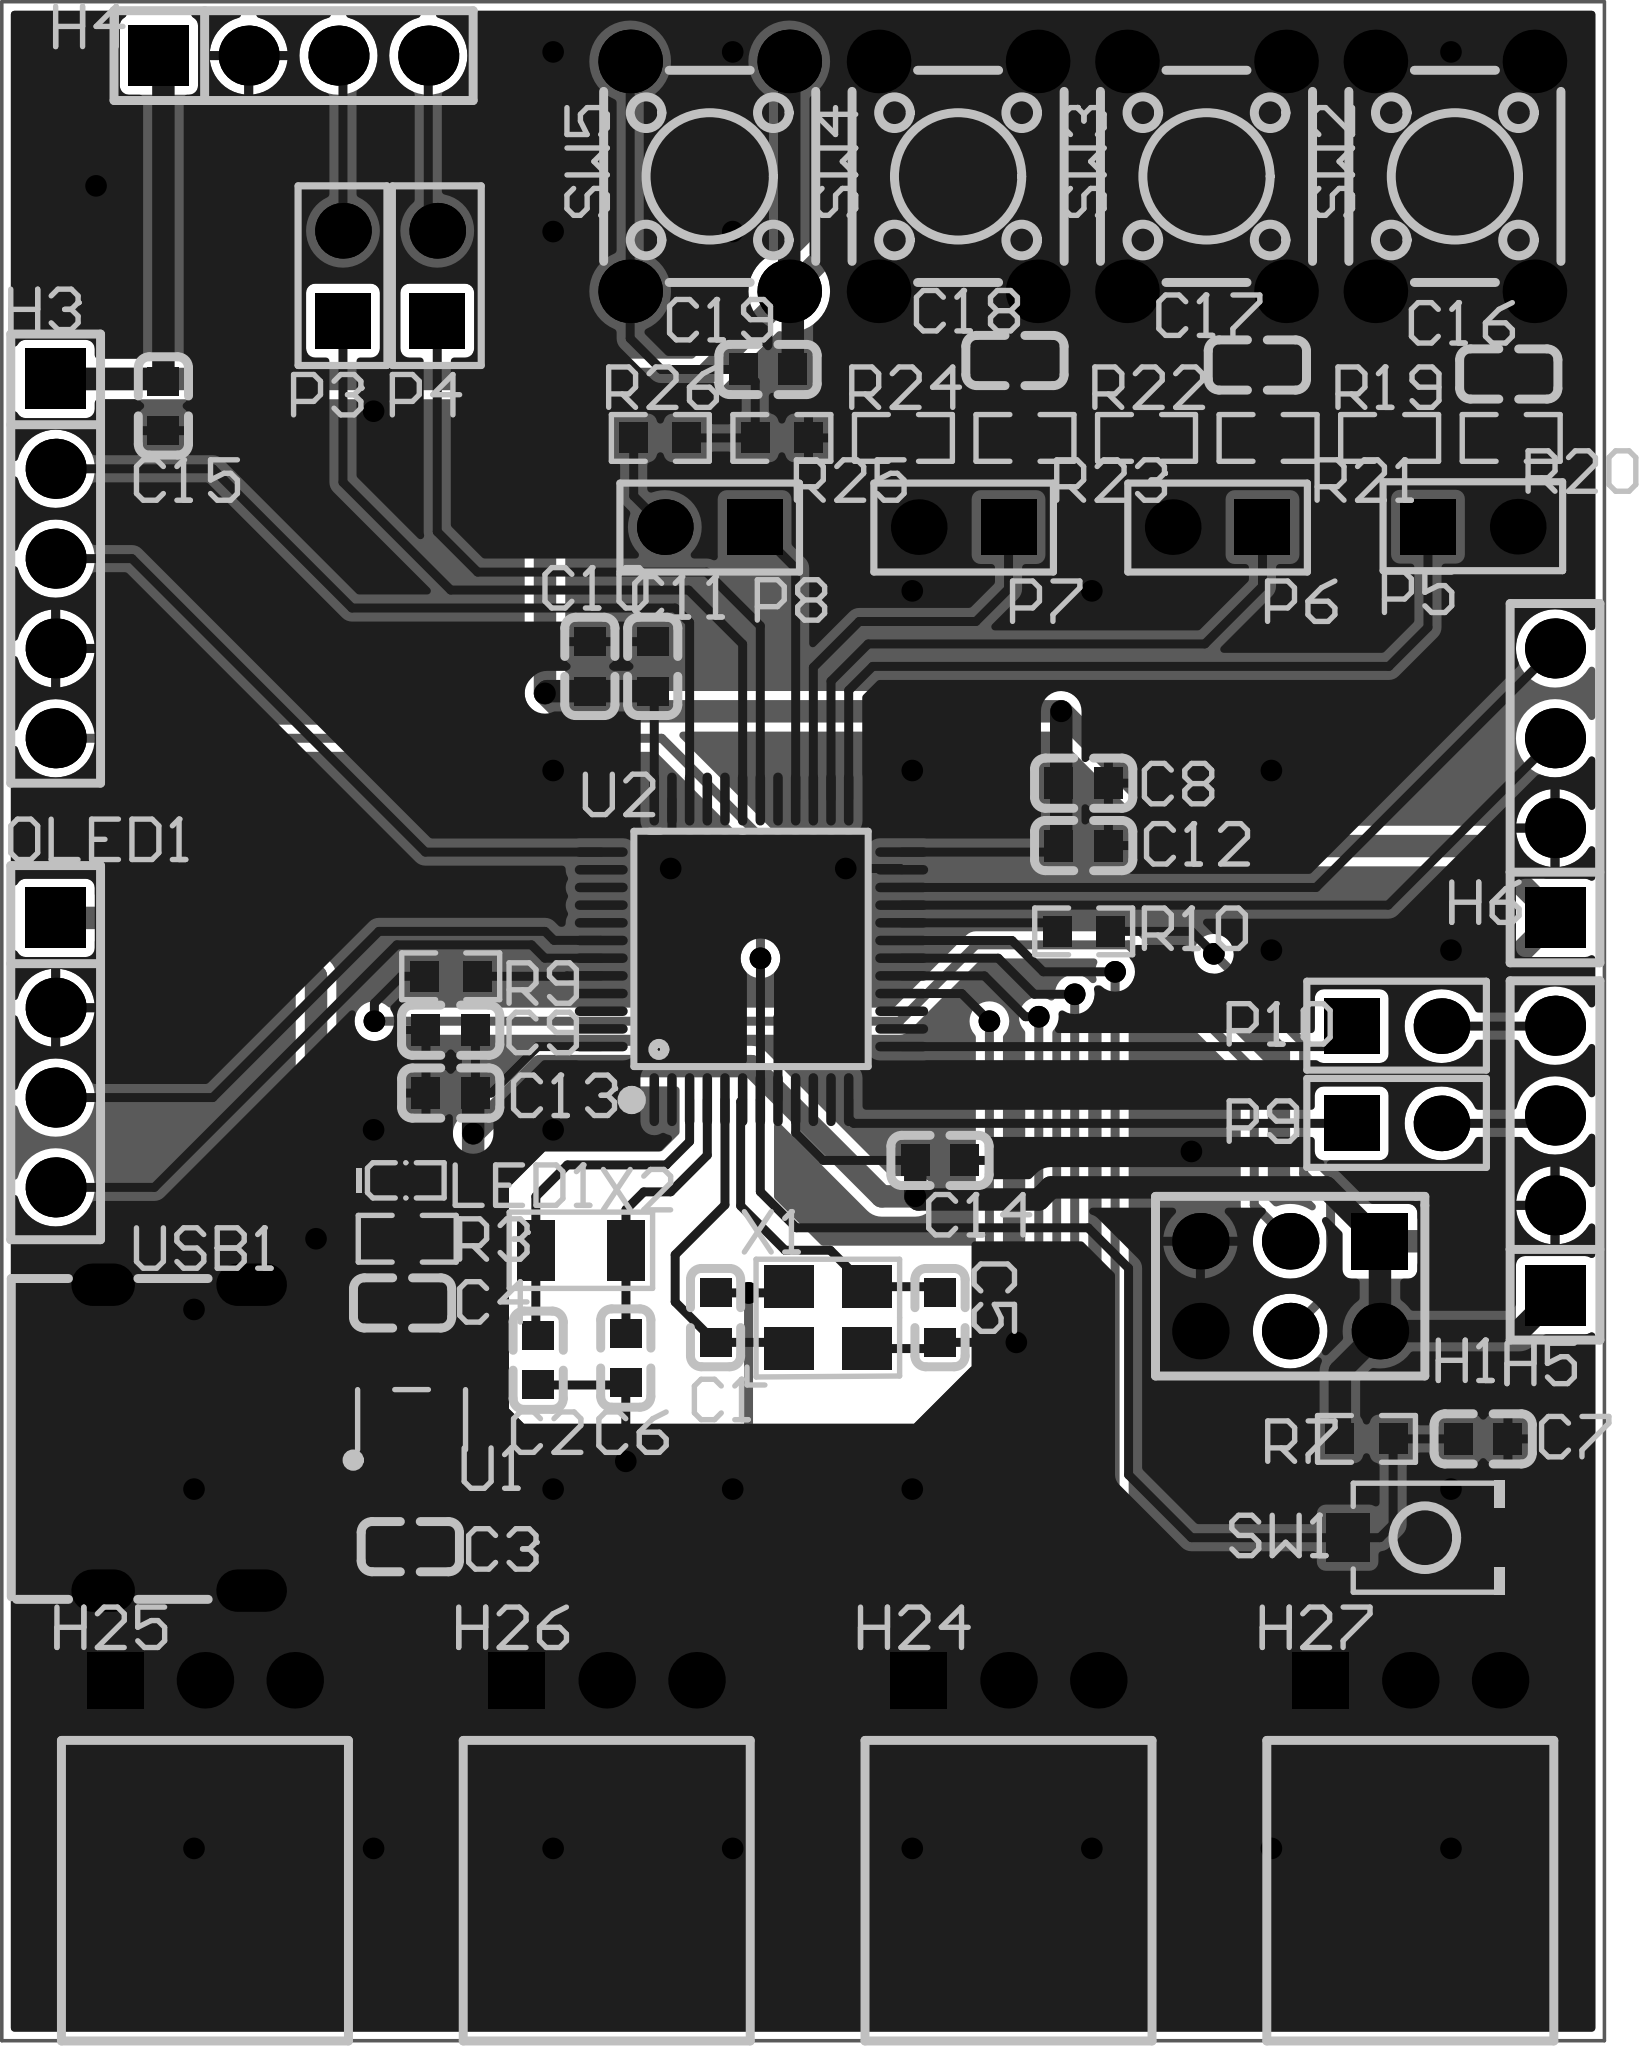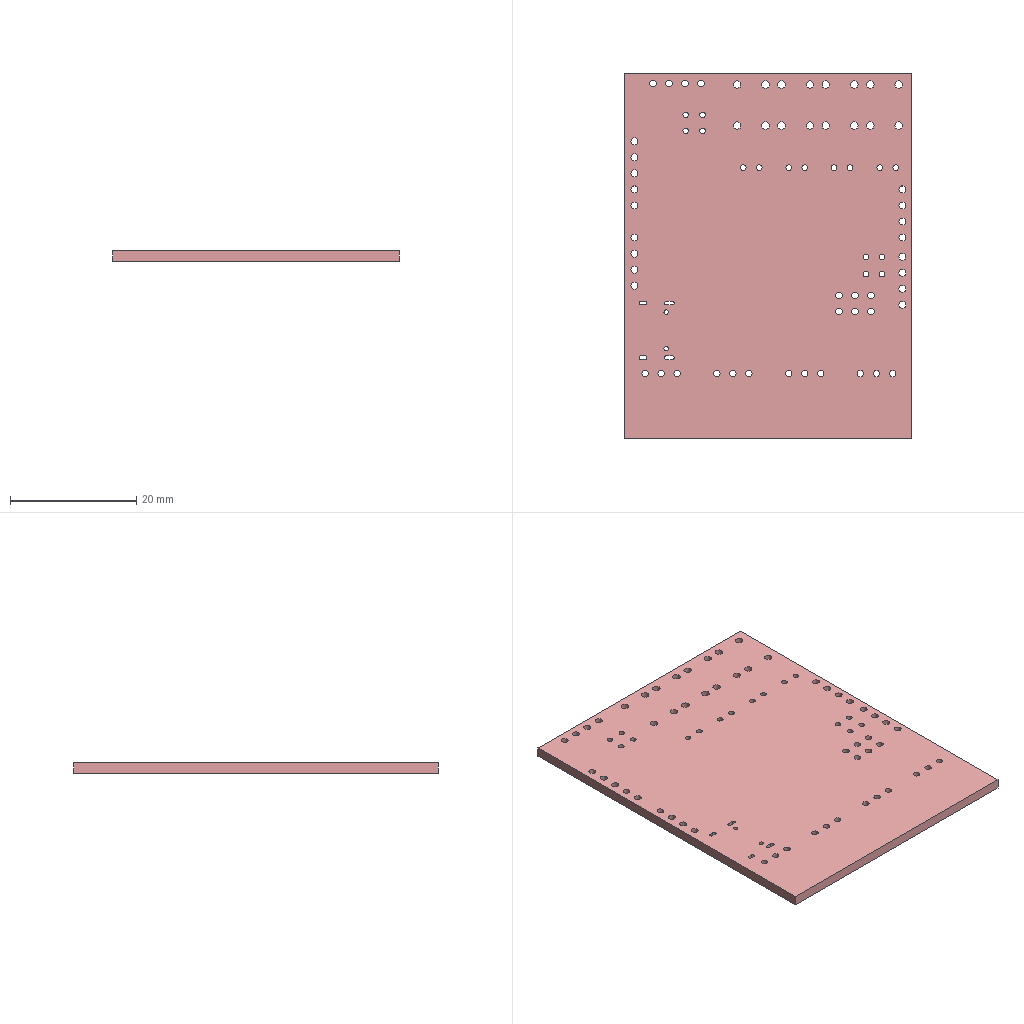Circuit board layout | Altium Designer | box 45.3 x 57.7 x 1.6 mm
Layer stack:
# Altium Designer layer stack of  (unit mm; dielectric type: 0 none, 1 core, 2 prepreg, 3 surface material)
index,name,kind,layer,copper_thickness_mm,dielectric_type,dielectric_thickness_mm,dielectric_material,dielectric_constant
0,Top Paste Mask Layer,other,,,,,,
1,Top Silkscreen Layer,other,,,,,,
2,Top Solder Mask Layer,dielectric,,,3,0.01,,3.3
3,Top Layer,copper,Top Layer,0.035,,,,
4,Dielectric1,dielectric,,,3,1.51,FR4,4.5
5,Bottom Layer,copper,Bottom Layer,0.035,,,,
6,Bottom Solder Mask Layer,dielectric,,,3,0.01,,3.3
7,Bottom Silkscreen Layer,other,,,,,,
8,Bottom Paste Mask Layer,other,,,,,,
# drill layer pairs: low layer,high layer
drill_pair,Top Layer,Bottom Layer
Part placement:
Designator,Comment,Layer,Footprint,Center-X(mm),Center-Y(mm),Rotation
C1,18pF,TopLayer,C0603,104.013,102.235,90
C2,10pF,TopLayer,C0603,98.995,101.03,90
C3,1uF,TopLayer,C0603,95.377,95.758,180
C4,1uF,TopLayer,C0603,95.159,102.65,180
C5,18pF,TopLayer,C0603,110.363,102.235,270
C6,10pF,TopLayer,C0603,101.473,101.092,90
C7,1uF,TopLayer,C0603,125.73,98.806,0
C8,4.7uF,TopLayer,C0603,114.427,117.348,180
C9,100nF,TopLayer,C0603,96.52,110.363,180
C10,100nF,TopLayer,C0603,100.457,120.65,90
C11,100nF,TopLayer,C0603,102.235,120.65,270
C12,100nF,TopLayer,C0603,114.427,115.583,180
C13,100nF,TopLayer,C0603,96.52,108.585,0
C14,100nF,TopLayer,C0603,110.363,106.68,180
C15,100nF,TopLayer,C0603,88.392,128.016,90
C16,100nF,TopLayer,C0603,126.453,128.919,0
C17,100nF,TopLayer,C0603,119.341,129.173,0
C18,100nF,TopLayer,C0603,112.483,129.3,0
C19,100nF,TopLayer,C0603,105.498,129.046,0
H1,,TopLayer,HDR-TH_6P-P2.54-V-R2-C3-S2.54_A2541WV-2X3P,120.269,103.124,180
H3,PZ254V-11-05P,TopLayer,HDR-TH_5P-P2.54-V-M,85.344,123.698,270
H4,PZ254V-11-04P,TopLayer,HDR-TH_4P-P2.54-V-M,92.075,137.922,0
H5,PZ254V-11-04P,TopLayer,HDR-TH_4P-P2.54-V-M,127.762,106.68,90
H6,PZ254V-11-04P,TopLayer,HDR-TH_4P-P2.54-V-M,127.762,117.348,90
H24,HC-PM254-8.5H-1x3PW-02A,TopLayer,HDR-TH_3P-P2.54_HC-PM254-8.5H-1X3PW,112.301,91.98,0
H25,HC-PM254-8.5H-1x3PW-02A,TopLayer,HDR-TH_3P-P2.54_HC-PM254-8.5H-1X3PW,89.567,91.98,0
H26,HC-PM254-8.5H-1x3PW-02A,TopLayer,HDR-TH_3P-P2.54_HC-PM254-8.5H-1X3PW,100.934,91.98,0
H27,HC-PM254-8.5H-1x3PW-02A,TopLayer,HDR-TH_3P-P2.54_HC-PM254-8.5H-1X3PW,123.668,91.98,0
LED1,,TopLayer,LED_0402,95.249,106.117,0
OLED1,2.54-1*4P female,TopLayer,HDR-TH_4P-P2.54-V-F,85.344,109.728,270
P3,Jumper pin header,TopLayer,2P排针,93.472,131.699,90
P4,Jumper pin header,TopLayer,2P排针,96.139,131.699,90
P5,Jumper pin header,TopLayer,2P排针,125.437,124.601,0
P6,Jumper pin header,TopLayer,2P排针,118.216,124.589,180
P7,Jumper pin header,TopLayer,2P排针,111.031,124.589,180
P8,Jumper pin header,TopLayer,2P排针,103.847,124.589,180
P9,Jumper pin header,TopLayer,2P排针,123.28,107.728,0
P10,Jumper pin header,TopLayer,2P排针,123.28,110.478,0
R3,1kΩ,TopLayer,R0603,95.29,104.466,0
R7,10kΩ,TopLayer,R0603,122.428,98.806,180
R9,10kΩ,TopLayer,R0603,96.52,111.887,180
R10,10kΩ,TopLayer,R0603,114.427,113.157,180
R19,4.7kΩ,TopLayer,R0603,123.083,127.111,0
R20,1kΩ,TopLayer,R0603,126.522,127.111,180
R21,4.7kΩ,TopLayer,R0603,119.644,127.111,180
R22,1kΩ,TopLayer,R0603,116.205,127.111,0
R23,4.7kΩ,TopLayer,R0603,112.766,127.111,180
R24,1kΩ,TopLayer,R0603,109.328,127.111,0
R25,4.7kΩ,TopLayer,R0603,105.889,127.111,180
R26,1kΩ,TopLayer,R0603,102.45,127.111,0
SW1,TS-1088-AR02016,TopLayer,SW-SMD_L3.9-W3.0-P4.45,124.079,96.012,0
SW2,TS665CJ,TopLayer,SW-TH_4P-L6.0-W6.0-P4.50-LS6.5,124.929,134.507,90
SW3,TS665CJ,TopLayer,SW-TH_4P-L6.0-W6.0-P4.50-LS6.5,117.902,134.507,90
SW4,TS665CJ,TopLayer,SW-TH_4P-L6.0-W6.0-P4.50-LS6.5,110.874,134.507,90
SW5,TS665CJ,TopLayer,SW-TH_4P-L6.0-W6.0-P4.50-LS6.5,103.847,134.507,90
U1,ME6211C33M5G-N,TopLayer,SOT-23-5_L3.0-W1.7-P0.95-LS2.8-BL,95.413,99.349,0
U2,STM32F103C8T6,TopLayer,LQFP-48_L7.0-W7.0-P0.50-LS9.0-BL,105.029,112.649,0
USB1,TYPE-C 16PIN 2MD(073),TopLayer,USB-C-SMD_TYPE-C-6PIN-2MD-073,89.063,98.841,270
X1,8MHz,TopLayer,OSC-SMD_4P-L3.2-W2.5-BL,107.188,102.235,0
X2,32.768kHz,TopLayer,CRYSTAL-SMD_L3.2-W1.5-1,100.203,104.14,180
Pad and via stacks:
# Altium Designer via and pad stacks of  (unit mm). Each distinct definition once, with the count of objects using it.
# via: kind,start_layer,end_layer,hole_mm,diameter_mm,mode(0 simple;1 top-mid-bottom;2 full stack),diameter_per_layer,count,example_net
# pad: kind,layer,hole_mm,hole_type(0 round;1 square;2 slot),plating,top_size,top_shape(1 round;2 rect;3 octagon;9 rounded rect),mid_size,bottom_size,mode,footprint,size_per_layer,count,example
pad,Top Layer,0,0,plated,0.8x0.9,2,0.8x0.9,0.8x0.9,0,C0603,,38,C1.2
pad,Top Layer,0,0,plated,0.6375x0.541,2,0.6375x0.541,0.6375x0.541,0,LED_0402,,2,LED1.2
pad,Top Layer,0,0,plated,0.8065x0.864,2,0.8065x0.864,0.8065x0.864,0,R0603,,24,R3.2
pad,Top Layer,0,0,plated,1.23x1.36,2,1.23x1.36,1.23x1.36,0,SW-SMD_L3.9-W3.0-P4.45,,2,SW1.1
pad,Top Layer,0,0,plated,0.49x1.157,2,0.49x1.157,0.49x1.157,0,SOT-23-5_L3.0-W1.7-P0.95-LS2.8-BL,,3,U1.1
pad,Top Layer,0,0,plated,0.49x1.175,2,0.49x1.175,0.49x1.175,0,SOT-23-5_L3.0-W1.7-P0.95-LS2.8-BL,,2,U1.4
pad,Top Layer,0,0,plated,0.27x1.5,1,0.27x1.5,0.27x1.5,0,LQFP-48_L7.0-W7.0-P0.50-LS9.0-BL,,24,U2.1
pad,Top Layer,0,0,plated,1.5x0.27,1,1.5x0.27,1.5x0.27,0,LQFP-48_L7.0-W7.0-P0.50-LS9.0-BL,,24,U2.13
pad,Top Layer,0,0,plated,0.6x1.1,2,0.6x1.1,0.6x1.1,0,USB-C-SMD_TYPE-C-6PIN-2MD-073,,4,USB1.1
pad,Top Layer,0,0,plated,0.3x1.1,2,0.3x1.1,0.3x1.1,0,USB-C-SMD_TYPE-C-6PIN-2MD-073,,8,USB1.3
pad,Top Layer,0,0,plated,1.4x1.2,2,1.4x1.2,1.4x1.2,0,OSC-SMD_4P-L3.2-W2.5-BL,,4,X1.1
pad,Top Layer,0,0,plated,1.05x1.7,2,1.05x1.7,1.05x1.7,0,CRYSTAL-SMD_L3.2-W1.5-1,,2,X2.2
pad,Multi-Layer,1.05,0,plated,1.6x1.6,2,1.6x1.6,1.6x1.6,0,HDR-TH_6P-P2.54-V-R2-C3-S2.54_A2541WV-2X3P,,1,H1.1
pad,Multi-Layer,1.05,0,plated,1.6x1.6,1,1.6x1.6,1.6x1.6,0,HDR-TH_6P-P2.54-V-R2-C3-S2.54_A2541WV-2X3P,,5,H1.2
pad,Multi-Layer,1.1,0,plated,1.7x1.7,2,1.7x1.7,1.7x1.7,0,HDR-TH_5P-P2.54-V-M,,1,H3.1
pad,Multi-Layer,1.1,0,plated,1.7x1.7,1,1.7x1.7,1.7x1.7,0,HDR-TH_5P-P2.54-V-M,,4,H3.2
pad,Multi-Layer,1.1,0,plated,1.7x1.7,2,1.7x1.7,1.7x1.7,0,HDR-TH_4P-P2.54-V-M,,3,H4.1
pad,Multi-Layer,1.1,0,plated,1.7x1.7,1,1.7x1.7,1.7x1.7,0,HDR-TH_4P-P2.54-V-M,,9,H4.2
pad,Multi-Layer,1.02,0,plated,1.6x1.6,2,1.6x1.6,1.6x1.6,0,HDR-TH_3P-P2.54_HC-PM254-8.5H-1X3PW,,4,H24.1
pad,Multi-Layer,1.02,0,plated,1.6x1.6,1,1.6x1.6,1.6x1.6,0,HDR-TH_3P-P2.54_HC-PM254-8.5H-1X3PW,,8,H24.2
pad,Multi-Layer,1.1,0,plated,1.7x1.7,2,1.7x1.7,1.7x1.7,0,HDR-TH_4P-P2.54-V-F,,1,OLED1.1
pad,Multi-Layer,1.1,0,plated,1.7x1.7,1,1.7x1.7,1.7x1.7,0,HDR-TH_4P-P2.54-V-F,,3,OLED1.2
pad,Multi-Layer,0.889,0,plated,1.575x1.575,2,1.575x1.575,1.575x1.575,0,2P\u00C5\u00C5\u00D5\u00EB,,8,P3.1
pad,Multi-Layer,0.889,0,plated,1.575x1.575,1,1.575x1.575,1.575x1.575,0,2P\u00C5\u00C5\u00D5\u00EB,,8,P3.2
pad,Multi-Layer,1.2,0,plated,1.8x1.8,1,1.8x1.8,1.8x1.8,0,SW-TH_4P-L6.0-W6.0-P4.50-LS6.5,,16,SW2.1
pad,Multi-Layer,0.6,2,plated,1.2x2,1,1.2x2,1.2x2,0,USB-C-SMD_TYPE-C-6PIN-2MD-073,,2,USB1.13
pad,Multi-Layer,0.6,2,plated,1.2x1.8,1,1.2x1.8,1.2x1.8,0,USB-C-SMD_TYPE-C-6PIN-2MD-073,,2,USB1.13
via,Top Layer,Bottom Layer,0.3048,0.61,0,,48,$1N5490
Copper pours:
name,layer,net,type(0 solid;1 hatched;2 none)
Bottom Layer-GND,Bottom Layer,GND,0
Top Layer-GND,Top Layer,GND,0